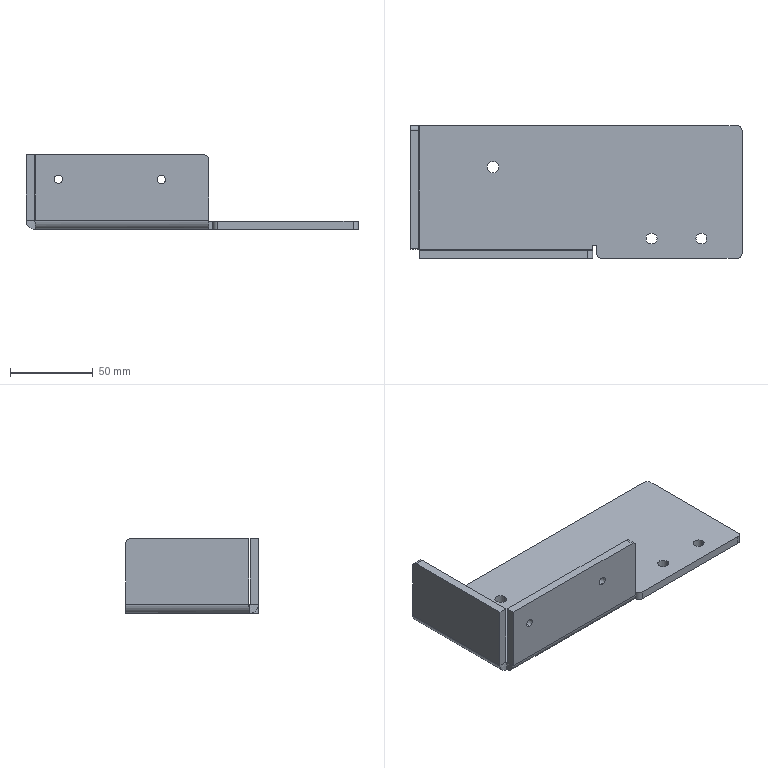Part | SolidWorks | features HoleWzd 3, EdgeFlange 1, Fillet 1, FlatPattern 1, SMBaseFlange 1, SheetMetal 1 | 1 solid | 41 faces | box 200 x 80 x 45 mm | volume 113530 mm3 | plane 20 | cylinder 19 | spline 2 | commonest cylinder face diameters 6 x5 5 x4 6.6 x4 1 x2 7 x2 11 x2
STEP:
#1=CARTESIAN_POINT('',(-18.5,-35.,22.5));
#2=VERTEX_POINT('',#1);
#3=CARTESIAN_POINT('',(-18.5,-35.,27.5));
#4=VERTEX_POINT('',#3);
#5=CARTESIAN_POINT('',(-18.5,-35.,25.));
#6=DIRECTION('',(0.,1.,0.));
#7=DIRECTION('',(0.,0.,1.));
#8=AXIS2_PLACEMENT_3D('',#5,#6,#7);
#9=CIRCLE('',#8,2.5);
#10=EDGE_CURVE('',#2,#4,#9,.T.);
#11=ORIENTED_EDGE('',*,*,#10,.T.);
#12=CARTESIAN_POINT('',(-18.5,-40.,27.5));
#13=VERTEX_POINT('',#12);
#14=CARTESIAN_POINT('',(-18.5,-40.,27.5));
#15=DIRECTION('',(0.,-1.,0.));
#16=VECTOR('',#15,1000.);
#17=LINE('',#14,#16);
#18=EDGE_CURVE('',#4,#13,#17,.T.);
#19=ORIENTED_EDGE('',*,*,#18,.T.);
#20=CARTESIAN_POINT('',(-18.5,-40.,22.5));
#21=VERTEX_POINT('',#20);
#22=CARTESIAN_POINT('',(-18.5,-40.,25.));
#23=DIRECTION('',(0.,-1.,0.));
#24=DIRECTION('',(0.,0.,-1.));
#25=AXIS2_PLACEMENT_3D('',#22,#23,#24);
#26=CIRCLE('',#25,2.5);
#27=EDGE_CURVE('',#13,#21,#26,.T.);
#28=ORIENTED_EDGE('',*,*,#27,.T.);
#29=CARTESIAN_POINT('',(-18.5,-40.,22.5));
#30=DIRECTION('',(0.,-1.,0.));
#31=VECTOR('',#30,1000.);
#32=LINE('',#29,#31);
#33=EDGE_CURVE('',#2,#21,#32,.T.);
#34=ORIENTED_EDGE('',*,*,#33,.F.);
#35=EDGE_LOOP('',(#11,#19,#28,#34));
#36=FACE_OUTER_BOUND('',#35,.T.);
#37=CARTESIAN_POINT('',(-18.5,-40.,25.));
#38=DIRECTION('',(0.,-1.,0.));
#39=DIRECTION('',(0.,0.,-1.));
#40=AXIS2_PLACEMENT_3D('',#37,#38,#39);
#41=CYLINDRICAL_SURFACE('',#40,2.5);
#42=ADVANCED_FACE('',(#36),#41,.F.);
#43=CARTESIAN_POINT('',(-80.5,-35.,22.646));
#44=VERTEX_POINT('',#43);
#45=CARTESIAN_POINT('',(-80.5,-35.,27.646));
#46=VERTEX_POINT('',#45);
#47=CARTESIAN_POINT('',(-80.5,-35.,25.146));
#48=DIRECTION('',(0.,1.,0.));
#49=DIRECTION('',(0.,0.,1.));
#50=AXIS2_PLACEMENT_3D('',#47,#48,#49);
#51=CIRCLE('',#50,2.5);
#52=EDGE_CURVE('',#44,#46,#51,.T.);
#53=ORIENTED_EDGE('',*,*,#52,.T.);
#54=CARTESIAN_POINT('',(-80.5,-40.,27.646));
#55=VERTEX_POINT('',#54);
#56=CARTESIAN_POINT('',(-80.5,-40.,27.646));
#57=DIRECTION('',(0.,-1.,0.));
#58=VECTOR('',#57,1000.);
#59=LINE('',#56,#58);
#60=EDGE_CURVE('',#46,#55,#59,.T.);
#61=ORIENTED_EDGE('',*,*,#60,.T.);
#62=CARTESIAN_POINT('',(-80.5,-40.,22.646));
#63=VERTEX_POINT('',#62);
#64=CARTESIAN_POINT('',(-80.5,-40.,25.146));
#65=DIRECTION('',(0.,-1.,0.));
#66=DIRECTION('',(0.,0.,-1.));
#67=AXIS2_PLACEMENT_3D('',#64,#65,#66);
#68=CIRCLE('',#67,2.5);
#69=EDGE_CURVE('',#55,#63,#68,.T.);
#70=ORIENTED_EDGE('',*,*,#69,.T.);
#71=CARTESIAN_POINT('',(-80.5,-40.,22.646));
#72=DIRECTION('',(0.,-1.,0.));
#73=VECTOR('',#72,1000.);
#74=LINE('',#71,#73);
#75=EDGE_CURVE('',#44,#63,#74,.T.);
#76=ORIENTED_EDGE('',*,*,#75,.F.);
#77=EDGE_LOOP('',(#53,#61,#70,#76));
#78=FACE_OUTER_BOUND('',#77,.T.);
#79=CARTESIAN_POINT('',(-80.5,-40.,25.146));
#80=DIRECTION('',(0.,-1.,0.));
#81=DIRECTION('',(0.,0.,-1.));
#82=AXIS2_PLACEMENT_3D('',#79,#80,#81);
#83=CYLINDRICAL_SURFACE('',#82,2.5);
#84=ADVANCED_FACE('',(#78),#83,.F.);
#85=CARTESIAN_POINT('',(-53.5,15.,-5.));
#86=VERTEX_POINT('',#85);
#87=CARTESIAN_POINT('',(-46.5,15.,-5.));
#88=VERTEX_POINT('',#87);
#89=CARTESIAN_POINT('',(-50.,15.,-5.));
#90=DIRECTION('',(0.,0.,1.));
#91=DIRECTION('',(1.,0.,0.));
#92=AXIS2_PLACEMENT_3D('',#89,#90,#91);
#93=CIRCLE('',#92,3.5);
#94=EDGE_CURVE('',#86,#88,#93,.T.);
#95=ORIENTED_EDGE('',*,*,#94,.F.);
#96=CARTESIAN_POINT('',(-53.5,15.,0.));
#97=VERTEX_POINT('',#96);
#98=CARTESIAN_POINT('',(-53.5,15.,0.));
#99=DIRECTION('',(0.,0.,1.));
#100=VECTOR('',#99,1000.);
#101=LINE('',#98,#100);
#102=EDGE_CURVE('',#86,#97,#101,.T.);
#103=ORIENTED_EDGE('',*,*,#102,.T.);
#104=CARTESIAN_POINT('',(-46.5,15.,0.));
#105=VERTEX_POINT('',#104);
#106=CARTESIAN_POINT('',(-50.,15.,0.));
#107=DIRECTION('',(0.,0.,1.));
#108=DIRECTION('',(1.,0.,0.));
#109=AXIS2_PLACEMENT_3D('',#106,#107,#108);
#110=CIRCLE('',#109,3.5);
#111=EDGE_CURVE('',#97,#105,#110,.T.);
#112=ORIENTED_EDGE('',*,*,#111,.T.);
#113=CARTESIAN_POINT('',(-46.5,15.,0.));
#114=DIRECTION('',(0.,0.,1.));
#115=VECTOR('',#114,1000.);
#116=LINE('',#113,#115);
#117=EDGE_CURVE('',#88,#105,#116,.T.);
#118=ORIENTED_EDGE('',*,*,#117,.F.);
#119=EDGE_LOOP('',(#95,#103,#112,#118));
#120=FACE_OUTER_BOUND('',#119,.T.);
#121=CARTESIAN_POINT('',(-50.,15.,0.));
#122=DIRECTION('',(0.,0.,1.));
#123=DIRECTION('',(1.,0.,0.));
#124=AXIS2_PLACEMENT_3D('',#121,#122,#123);
#125=CYLINDRICAL_SURFACE('',#124,3.5);
#126=ADVANCED_FACE('',(#120),#125,.F.);
#127=CARTESIAN_POINT('',(72.2,-28.,-5.));
#128=VERTEX_POINT('',#127);
#129=CARTESIAN_POINT('',(78.8,-28.,-5.));
#130=VERTEX_POINT('',#129);
#131=CARTESIAN_POINT('',(75.5,-28.,-5.));
#132=DIRECTION('',(0.,0.,1.));
#133=DIRECTION('',(1.,0.,0.));
#134=AXIS2_PLACEMENT_3D('',#131,#132,#133);
#135=CIRCLE('',#134,3.3);
#136=EDGE_CURVE('',#128,#130,#135,.T.);
#137=ORIENTED_EDGE('',*,*,#136,.F.);
#138=CARTESIAN_POINT('',(72.2,-28.,0.));
#139=VERTEX_POINT('',#138);
#140=CARTESIAN_POINT('',(72.2,-28.,0.));
#141=DIRECTION('',(0.,0.,1.));
#142=VECTOR('',#141,1000.);
#143=LINE('',#140,#142);
#144=EDGE_CURVE('',#128,#139,#143,.T.);
#145=ORIENTED_EDGE('',*,*,#144,.T.);
#146=CARTESIAN_POINT('',(78.8,-28.,0.));
#147=VERTEX_POINT('',#146);
#148=CARTESIAN_POINT('',(75.5,-28.,0.));
#149=DIRECTION('',(0.,0.,1.));
#150=DIRECTION('',(1.,0.,0.));
#151=AXIS2_PLACEMENT_3D('',#148,#149,#150);
#152=CIRCLE('',#151,3.3);
#153=EDGE_CURVE('',#139,#147,#152,.T.);
#154=ORIENTED_EDGE('',*,*,#153,.T.);
#155=CARTESIAN_POINT('',(78.8,-28.,0.));
#156=DIRECTION('',(0.,0.,1.));
#157=VECTOR('',#156,1000.);
#158=LINE('',#155,#157);
#159=EDGE_CURVE('',#130,#147,#158,.T.);
#160=ORIENTED_EDGE('',*,*,#159,.F.);
#161=EDGE_LOOP('',(#137,#145,#154,#160));
#162=FACE_OUTER_BOUND('',#161,.T.);
#163=CARTESIAN_POINT('',(75.5,-28.,0.));
#164=DIRECTION('',(0.,0.,1.));
#165=DIRECTION('',(1.,0.,0.));
#166=AXIS2_PLACEMENT_3D('',#163,#164,#165);
#167=CYLINDRICAL_SURFACE('',#166,3.3);
#168=ADVANCED_FACE('',(#162),#167,.F.);
#169=CARTESIAN_POINT('',(42.2,-28.,-5.));
#170=VERTEX_POINT('',#169);
#171=CARTESIAN_POINT('',(48.8,-28.,-5.));
#172=VERTEX_POINT('',#171);
#173=CARTESIAN_POINT('',(45.5,-28.,-5.));
#174=DIRECTION('',(0.,0.,1.));
#175=DIRECTION('',(1.,0.,0.));
#176=AXIS2_PLACEMENT_3D('',#173,#174,#175);
#177=CIRCLE('',#176,3.3);
#178=EDGE_CURVE('',#170,#172,#177,.T.);
#179=ORIENTED_EDGE('',*,*,#178,.F.);
#180=CARTESIAN_POINT('',(42.2,-28.,0.));
#181=VERTEX_POINT('',#180);
#182=CARTESIAN_POINT('',(42.2,-28.,0.));
#183=DIRECTION('',(0.,0.,1.));
#184=VECTOR('',#183,1000.);
#185=LINE('',#182,#184);
#186=EDGE_CURVE('',#170,#181,#185,.T.);
#187=ORIENTED_EDGE('',*,*,#186,.T.);
#188=CARTESIAN_POINT('',(48.8,-28.,0.));
#189=VERTEX_POINT('',#188);
#190=CARTESIAN_POINT('',(45.5,-28.,0.));
#191=DIRECTION('',(0.,0.,1.));
#192=DIRECTION('',(1.,0.,0.));
#193=AXIS2_PLACEMENT_3D('',#190,#191,#192);
#194=CIRCLE('',#193,3.3);
#195=EDGE_CURVE('',#181,#189,#194,.T.);
#196=ORIENTED_EDGE('',*,*,#195,.T.);
#197=CARTESIAN_POINT('',(48.8,-28.,0.));
#198=DIRECTION('',(0.,0.,1.));
#199=VECTOR('',#198,1000.);
#200=LINE('',#197,#199);
#201=EDGE_CURVE('',#172,#189,#200,.T.);
#202=ORIENTED_EDGE('',*,*,#201,.F.);
#203=EDGE_LOOP('',(#179,#187,#196,#202));
#204=FACE_OUTER_BOUND('',#203,.T.);
#205=CARTESIAN_POINT('',(45.5,-28.,0.));
#206=DIRECTION('',(0.,0.,1.));
#207=DIRECTION('',(1.,0.,0.));
#208=AXIS2_PLACEMENT_3D('',#205,#206,#207);
#209=CYLINDRICAL_SURFACE('',#208,3.3);
#210=ADVANCED_FACE('',(#204),#209,.F.);
#211=CARTESIAN_POINT('',(-50.,15.,-5.));
#212=DIRECTION('',(0.,0.,1.));
#213=DIRECTION('',(1.,0.,0.));
#214=AXIS2_PLACEMENT_3D('',#211,#212,#213);
#215=CIRCLE('',#214,3.5);
#216=EDGE_CURVE('',#88,#86,#215,.T.);
#217=ORIENTED_EDGE('',*,*,#216,.T.);
#218=ORIENTED_EDGE('',*,*,#94,.T.);
#219=EDGE_LOOP('',(#217,#218));
#220=FACE_BOUND('',#219,.T.);
#221=CARTESIAN_POINT('',(75.5,-28.,-5.));
#222=DIRECTION('',(0.,0.,1.));
#223=DIRECTION('',(1.,0.,0.));
#224=AXIS2_PLACEMENT_3D('',#221,#222,#223);
#225=CIRCLE('',#224,3.3);
#226=EDGE_CURVE('',#130,#128,#225,.T.);
#227=ORIENTED_EDGE('',*,*,#226,.T.);
#228=ORIENTED_EDGE('',*,*,#136,.T.);
#229=EDGE_LOOP('',(#227,#228));
#230=FACE_BOUND('',#229,.T.);
#231=CARTESIAN_POINT('',(45.5,-28.,-5.));
#232=DIRECTION('',(0.,0.,1.));
#233=DIRECTION('',(1.,0.,0.));
#234=AXIS2_PLACEMENT_3D('',#231,#232,#233);
#235=CIRCLE('',#234,3.3);
#236=EDGE_CURVE('',#172,#170,#235,.T.);
#237=ORIENTED_EDGE('',*,*,#236,.T.);
#238=ORIENTED_EDGE('',*,*,#178,.T.);
#239=EDGE_LOOP('',(#237,#238));
#240=FACE_BOUND('',#239,.T.);
#241=CARTESIAN_POINT('',(15.5,-40.,-5.));
#242=VERTEX_POINT('',#241);
#243=CARTESIAN_POINT('',(97.,-40.,-5.));
#244=VERTEX_POINT('',#243);
#245=CARTESIAN_POINT('',(100.,-40.,-5.));
#246=DIRECTION('',(1.,0.,0.));
#247=VECTOR('',#246,1000.);
#248=LINE('',#245,#247);
#249=EDGE_CURVE('',#242,#244,#248,.T.);
#250=ORIENTED_EDGE('',*,*,#249,.F.);
#251=CARTESIAN_POINT('',(12.5,-37.,-5.));
#252=VERTEX_POINT('',#251);
#253=CARTESIAN_POINT('',(15.5,-37.,-5.));
#254=DIRECTION('',(0.,0.,-1.));
#255=DIRECTION('',(1.,0.,0.));
#256=AXIS2_PLACEMENT_3D('',#253,#254,#255);
#257=CIRCLE('',#256,3.);
#258=EDGE_CURVE('',#242,#252,#257,.T.);
#259=ORIENTED_EDGE('',*,*,#258,.T.);
#260=CARTESIAN_POINT('',(12.5,-32.,-5.));
#261=VERTEX_POINT('',#260);
#262=CARTESIAN_POINT('',(12.5,0.,-5.));
#263=DIRECTION('',(0.,-1.,0.));
#264=VECTOR('',#263,1000.);
#265=LINE('',#262,#264);
#266=EDGE_CURVE('',#261,#252,#265,.T.);
#267=ORIENTED_EDGE('',*,*,#266,.F.);
#268=CARTESIAN_POINT('',(10.,-32.,-5.));
#269=VERTEX_POINT('',#268);
#270=CARTESIAN_POINT('',(0.,-32.,-5.));
#271=DIRECTION('',(1.,0.,0.));
#272=VECTOR('',#271,1000.);
#273=LINE('',#270,#272);
#274=EDGE_CURVE('',#269,#261,#273,.T.);
#275=ORIENTED_EDGE('',*,*,#274,.F.);
#276=CARTESIAN_POINT('',(10.,-34.5,-5.));
#277=VERTEX_POINT('',#276);
#278=CARTESIAN_POINT('',(10.,0.,-5.));
#279=DIRECTION('',(0.,1.,0.));
#280=VECTOR('',#279,1000.);
#281=LINE('',#278,#280);
#282=EDGE_CURVE('',#277,#269,#281,.T.);
#283=ORIENTED_EDGE('',*,*,#282,.F.);
#284=CARTESIAN_POINT('',(-94.5,-34.5,-5.));
#285=VERTEX_POINT('',#284);
#286=CARTESIAN_POINT('',(10.,-34.5,-5.));
#287=DIRECTION('',(-1.,0.,0.));
#288=VECTOR('',#287,1000.);
#289=LINE('',#286,#288);
#290=EDGE_CURVE('',#277,#285,#289,.T.);
#291=ORIENTED_EDGE('',*,*,#290,.T.);
#292=CARTESIAN_POINT('',(-94.5,40.,-5.));
#293=VERTEX_POINT('',#292);
#294=CARTESIAN_POINT('',(-94.5,-34.5,-5.));
#295=DIRECTION('',(0.,1.,0.));
#296=VECTOR('',#295,1000.);
#297=LINE('',#294,#296);
#298=EDGE_CURVE('',#285,#293,#297,.T.);
#299=ORIENTED_EDGE('',*,*,#298,.T.);
#300=CARTESIAN_POINT('',(97.,40.,-5.));
#301=VERTEX_POINT('',#300);
#302=CARTESIAN_POINT('',(100.,40.,-5.));
#303=DIRECTION('',(-1.,0.,0.));
#304=VECTOR('',#303,1000.);
#305=LINE('',#302,#304);
#306=EDGE_CURVE('',#301,#293,#305,.T.);
#307=ORIENTED_EDGE('',*,*,#306,.F.);
#308=CARTESIAN_POINT('',(100.,37.,-5.));
#309=VERTEX_POINT('',#308);
#310=CARTESIAN_POINT('',(97.,37.,-5.));
#311=DIRECTION('',(0.,0.,-1.));
#312=DIRECTION('',(1.,0.,0.));
#313=AXIS2_PLACEMENT_3D('',#310,#311,#312);
#314=CIRCLE('',#313,3.);
#315=EDGE_CURVE('',#301,#309,#314,.T.);
#316=ORIENTED_EDGE('',*,*,#315,.T.);
#317=CARTESIAN_POINT('',(100.,-37.,-5.));
#318=VERTEX_POINT('',#317);
#319=CARTESIAN_POINT('',(100.,-40.,-5.));
#320=DIRECTION('',(0.,1.,0.));
#321=VECTOR('',#320,1000.);
#322=LINE('',#319,#321);
#323=EDGE_CURVE('',#318,#309,#322,.T.);
#324=ORIENTED_EDGE('',*,*,#323,.F.);
#325=CARTESIAN_POINT('',(97.,-37.,-5.));
#326=DIRECTION('',(0.,0.,-1.));
#327=DIRECTION('',(1.,0.,0.));
#328=AXIS2_PLACEMENT_3D('',#325,#326,#327);
#329=CIRCLE('',#328,3.);
#330=EDGE_CURVE('',#318,#244,#329,.T.);
#331=ORIENTED_EDGE('',*,*,#330,.T.);
#332=EDGE_LOOP('',(#250,#259,#267,#275,#283,#291,#299,#307,#316,#324,#331));
#333=FACE_OUTER_BOUND('',#332,.T.);
#334=CARTESIAN_POINT('',(0.,0.,-5.));
#335=DIRECTION('',(0.,0.,1.));
#336=DIRECTION('',(1.,0.,0.));
#337=AXIS2_PLACEMENT_3D('',#334,#335,#336);
#338=PLANE('',#337);
#339=ADVANCED_FACE('',(#220,#230,#240,#333),#338,.F.);
#340=CARTESIAN_POINT('',(-50.,15.,0.));
#341=DIRECTION('',(0.,0.,1.));
#342=DIRECTION('',(1.,0.,0.));
#343=AXIS2_PLACEMENT_3D('',#340,#341,#342);
#344=CIRCLE('',#343,3.5);
#345=EDGE_CURVE('',#105,#97,#344,.T.);
#346=ORIENTED_EDGE('',*,*,#345,.F.);
#347=ORIENTED_EDGE('',*,*,#111,.F.);
#348=EDGE_LOOP('',(#346,#347));
#349=FACE_BOUND('',#348,.T.);
#350=CARTESIAN_POINT('',(75.5,-28.,0.));
#351=DIRECTION('',(0.,0.,1.));
#352=DIRECTION('',(1.,0.,0.));
#353=AXIS2_PLACEMENT_3D('',#350,#351,#352);
#354=CIRCLE('',#353,3.3);
#355=EDGE_CURVE('',#147,#139,#354,.T.);
#356=ORIENTED_EDGE('',*,*,#355,.F.);
#357=ORIENTED_EDGE('',*,*,#153,.F.);
#358=EDGE_LOOP('',(#356,#357));
#359=FACE_BOUND('',#358,.T.);
#360=CARTESIAN_POINT('',(45.5,-28.,0.));
#361=DIRECTION('',(0.,0.,1.));
#362=DIRECTION('',(1.,0.,0.));
#363=AXIS2_PLACEMENT_3D('',#360,#361,#362);
#364=CIRCLE('',#363,3.3);
#365=EDGE_CURVE('',#189,#181,#364,.T.);
#366=ORIENTED_EDGE('',*,*,#365,.F.);
#367=ORIENTED_EDGE('',*,*,#195,.F.);
#368=EDGE_LOOP('',(#366,#367));
#369=FACE_BOUND('',#368,.T.);
#370=CARTESIAN_POINT('',(12.5,-37.,0.));
#371=VERTEX_POINT('',#370);
#372=CARTESIAN_POINT('',(12.5,-32.,0.));
#373=VERTEX_POINT('',#372);
#374=CARTESIAN_POINT('',(12.5,-40.,0.));
#375=DIRECTION('',(0.,1.,0.));
#376=VECTOR('',#375,1000.);
#377=LINE('',#374,#376);
#378=EDGE_CURVE('',#371,#373,#377,.T.);
#379=ORIENTED_EDGE('',*,*,#378,.F.);
#380=CARTESIAN_POINT('',(15.5,-40.,0.));
#381=VERTEX_POINT('',#380);
#382=CARTESIAN_POINT('',(15.5,-37.,0.));
#383=DIRECTION('',(0.,0.,1.));
#384=DIRECTION('',(1.,0.,0.));
#385=AXIS2_PLACEMENT_3D('',#382,#383,#384);
#386=CIRCLE('',#385,3.);
#387=EDGE_CURVE('',#371,#381,#386,.T.);
#388=ORIENTED_EDGE('',*,*,#387,.T.);
#389=CARTESIAN_POINT('',(97.,-40.,0.));
#390=VERTEX_POINT('',#389);
#391=CARTESIAN_POINT('',(100.,-40.,0.));
#392=DIRECTION('',(1.,0.,0.));
#393=VECTOR('',#392,1000.);
#394=LINE('',#391,#393);
#395=EDGE_CURVE('',#381,#390,#394,.T.);
#396=ORIENTED_EDGE('',*,*,#395,.T.);
#397=CARTESIAN_POINT('',(100.,-37.,0.));
#398=VERTEX_POINT('',#397);
#399=CARTESIAN_POINT('',(97.,-37.,0.));
#400=DIRECTION('',(0.,0.,1.));
#401=DIRECTION('',(1.,0.,0.));
#402=AXIS2_PLACEMENT_3D('',#399,#400,#401);
#403=CIRCLE('',#402,3.);
#404=EDGE_CURVE('',#390,#398,#403,.T.);
#405=ORIENTED_EDGE('',*,*,#404,.T.);
#406=CARTESIAN_POINT('',(100.,37.,0.));
#407=VERTEX_POINT('',#406);
#408=CARTESIAN_POINT('',(100.,-40.,0.));
#409=DIRECTION('',(0.,1.,0.));
#410=VECTOR('',#409,1000.);
#411=LINE('',#408,#410);
#412=EDGE_CURVE('',#398,#407,#411,.T.);
#413=ORIENTED_EDGE('',*,*,#412,.T.);
#414=CARTESIAN_POINT('',(97.,40.,0.));
#415=VERTEX_POINT('',#414);
#416=CARTESIAN_POINT('',(97.,37.,0.));
#417=DIRECTION('',(0.,0.,1.));
#418=DIRECTION('',(1.,0.,0.));
#419=AXIS2_PLACEMENT_3D('',#416,#417,#418);
#420=CIRCLE('',#419,3.);
#421=EDGE_CURVE('',#407,#415,#420,.T.);
#422=ORIENTED_EDGE('',*,*,#421,.T.);
#423=CARTESIAN_POINT('',(-94.5,40.,0.));
#424=VERTEX_POINT('',#423);
#425=CARTESIAN_POINT('',(100.,40.,0.));
#426=DIRECTION('',(-1.,0.,0.));
#427=VECTOR('',#426,1000.);
#428=LINE('',#425,#427);
#429=EDGE_CURVE('',#415,#424,#428,.T.);
#430=ORIENTED_EDGE('',*,*,#429,.T.);
#431=CARTESIAN_POINT('',(-94.5,-34.5,0.));
#432=VERTEX_POINT('',#431);
#433=CARTESIAN_POINT('',(-94.5,-34.5,0.));
#434=DIRECTION('',(0.,1.,0.));
#435=VECTOR('',#434,1000.);
#436=LINE('',#433,#435);
#437=EDGE_CURVE('',#432,#424,#436,.T.);
#438=ORIENTED_EDGE('',*,*,#437,.F.);
#439=CARTESIAN_POINT('',(10.,-34.5,0.));
#440=VERTEX_POINT('',#439);
#441=CARTESIAN_POINT('',(10.,-34.5,0.));
#442=DIRECTION('',(-1.,0.,0.));
#443=VECTOR('',#442,1000.);
#444=LINE('',#441,#443);
#445=EDGE_CURVE('',#440,#432,#444,.T.);
#446=ORIENTED_EDGE('',*,*,#445,.F.);
#447=CARTESIAN_POINT('',(10.,-32.,0.));
#448=VERTEX_POINT('',#447);
#449=CARTESIAN_POINT('',(10.,-32.,0.));
#450=DIRECTION('',(0.,-1.,0.));
#451=VECTOR('',#450,1000.);
#452=LINE('',#449,#451);
#453=EDGE_CURVE('',#448,#440,#452,.T.);
#454=ORIENTED_EDGE('',*,*,#453,.F.);
#455=CARTESIAN_POINT('',(12.5,-32.,0.));
#456=DIRECTION('',(-1.,0.,0.));
#457=VECTOR('',#456,1000.);
#458=LINE('',#455,#457);
#459=EDGE_CURVE('',#373,#448,#458,.T.);
#460=ORIENTED_EDGE('',*,*,#459,.F.);
#461=EDGE_LOOP('',(#379,#388,#396,#405,#413,#422,#430,#438,#446,#454,#460));
#462=FACE_OUTER_BOUND('',#461,.T.);
#463=CARTESIAN_POINT('',(0.,0.,0.));
#464=DIRECTION('',(0.,0.,1.));
#465=DIRECTION('',(1.,0.,0.));
#466=AXIS2_PLACEMENT_3D('',#463,#464,#465);
#467=PLANE('',#466);
#468=ADVANCED_FACE('',(#349,#359,#369,#462),#467,.T.);
#469=ORIENTED_EDGE('',*,*,#395,.F.);
#470=CARTESIAN_POINT('',(15.5,-40.,-5.));
#471=DIRECTION('',(0.,0.,-1.));
#472=VECTOR('',#471,1000.);
#473=LINE('',#470,#472);
#474=EDGE_CURVE('',#381,#242,#473,.T.);
#475=ORIENTED_EDGE('',*,*,#474,.T.);
#476=ORIENTED_EDGE('',*,*,#249,.T.);
#477=CARTESIAN_POINT('',(97.,-40.,-5.));
#478=DIRECTION('',(0.,0.,1.));
#479=VECTOR('',#478,1000.);
#480=LINE('',#477,#479);
#481=EDGE_CURVE('',#244,#390,#480,.T.);
#482=ORIENTED_EDGE('',*,*,#481,.T.);
#483=EDGE_LOOP('',(#469,#475,#476,#482));
#484=FACE_OUTER_BOUND('',#483,.T.);
#485=CARTESIAN_POINT('',(100.,-40.,-5.));
#486=DIRECTION('',(0.,-1.,0.));
#487=DIRECTION('',(1.,0.,0.));
#488=AXIS2_PLACEMENT_3D('',#485,#486,#487);
#489=PLANE('',#488);
#490=ADVANCED_FACE('',(#484),#489,.T.);
#491=ORIENTED_EDGE('',*,*,#429,.F.);
#492=CARTESIAN_POINT('',(97.,40.,-5.));
#493=DIRECTION('',(0.,0.,-1.));
#494=VECTOR('',#493,1000.);
#495=LINE('',#492,#494);
#496=EDGE_CURVE('',#415,#301,#495,.T.);
#497=ORIENTED_EDGE('',*,*,#496,.T.);
#498=ORIENTED_EDGE('',*,*,#306,.T.);
#499=CARTESIAN_POINT('',(-94.5,40.,0.));
#500=DIRECTION('',(0.,0.,-1.));
#501=VECTOR('',#500,1000.);
#502=LINE('',#499,#501);
#503=EDGE_CURVE('',#424,#293,#502,.T.);
#504=ORIENTED_EDGE('',*,*,#503,.F.);
#505=EDGE_LOOP('',(#491,#497,#498,#504));
#506=FACE_OUTER_BOUND('',#505,.T.);
#507=CARTESIAN_POINT('',(100.,40.,-5.));
#508=DIRECTION('',(0.,1.,0.));
#509=DIRECTION('',(-1.,0.,0.));
#510=AXIS2_PLACEMENT_3D('',#507,#508,#509);
#511=PLANE('',#510);
#512=ADVANCED_FACE('',(#506),#511,.T.);
#513=ORIENTED_EDGE('',*,*,#323,.T.);
#514=CARTESIAN_POINT('',(100.,37.,-5.));
#515=DIRECTION('',(0.,0.,1.));
#516=VECTOR('',#515,1000.);
#517=LINE('',#514,#516);
#518=EDGE_CURVE('',#309,#407,#517,.T.);
#519=ORIENTED_EDGE('',*,*,#518,.T.);
#520=ORIENTED_EDGE('',*,*,#412,.F.);
#521=CARTESIAN_POINT('',(100.,-37.,-5.));
#522=DIRECTION('',(0.,0.,-1.));
#523=VECTOR('',#522,1000.);
#524=LINE('',#521,#523);
#525=EDGE_CURVE('',#398,#318,#524,.T.);
#526=ORIENTED_EDGE('',*,*,#525,.T.);
#527=EDGE_LOOP('',(#513,#519,#520,#526));
#528=FACE_OUTER_BOUND('',#527,.T.);
#529=CARTESIAN_POINT('',(100.,-40.,-5.));
#530=DIRECTION('',(1.,0.,0.));
#531=DIRECTION('',(0.,0.,-1.));
#532=AXIS2_PLACEMENT_3D('',#529,#530,#531);
#533=PLANE('',#532);
#534=ADVANCED_FACE('',(#528),#533,.T.);
#535=ORIENTED_EDGE('',*,*,#266,.T.);
#536=CARTESIAN_POINT('',(12.5,-37.,0.));
#537=DIRECTION('',(0.,0.,1.));
#538=VECTOR('',#537,1000.);
#539=LINE('',#536,#538);
#540=EDGE_CURVE('',#252,#371,#539,.T.);
#541=ORIENTED_EDGE('',*,*,#540,.T.);
#542=ORIENTED_EDGE('',*,*,#378,.T.);
#543=CARTESIAN_POINT('',(12.5,-32.,0.));
#544=DIRECTION('',(0.,0.,-1.));
#545=VECTOR('',#544,1000.);
#546=LINE('',#543,#545);
#547=EDGE_CURVE('',#373,#261,#546,.T.);
#548=ORIENTED_EDGE('',*,*,#547,.T.);
#549=EDGE_LOOP('',(#535,#541,#542,#548));
#550=FACE_OUTER_BOUND('',#549,.T.);
#551=CARTESIAN_POINT('',(12.5,-40.,0.));
#552=DIRECTION('',(-1.,0.,0.));
#553=DIRECTION('',(0.,-1.,0.));
#554=AXIS2_PLACEMENT_3D('',#551,#552,#553);
#555=PLANE('',#554);
#556=ADVANCED_FACE('',(#550),#555,.T.);
#557=CARTESIAN_POINT('',(10.,-32.,0.));
#558=DIRECTION('',(0.,0.,-1.));
#559=VECTOR('',#558,1000.);
#560=LINE('',#557,#559);
#561=EDGE_CURVE('',#448,#269,#560,.T.);
#562=ORIENTED_EDGE('',*,*,#561,.T.);
#563=ORIENTED_EDGE('',*,*,#274,.T.);
#564=ORIENTED_EDGE('',*,*,#547,.F.);
#565=ORIENTED_EDGE('',*,*,#459,.T.);
#566=EDGE_LOOP('',(#562,#563,#564,#565));
#567=FACE_OUTER_BOUND('',#566,.T.);
#568=CARTESIAN_POINT('',(12.5,-32.,0.));
#569=DIRECTION('',(0.,-1.,0.));
#570=DIRECTION('',(0.,0.,-1.));
#571=AXIS2_PLACEMENT_3D('',#568,#569,#570);
#572=PLANE('',#571);
#573=ADVANCED_FACE('',(#567),#572,.T.);
#574=CARTESIAN_POINT('',(10.,-34.5,0.));
#575=DIRECTION('',(0.,0.,-1.));
#576=VECTOR('',#575,1000.);
#577=LINE('',#574,#576);
#578=EDGE_CURVE('',#440,#277,#577,.T.);
#579=ORIENTED_EDGE('',*,*,#578,.T.);
#580=ORIENTED_EDGE('',*,*,#282,.T.);
#581=ORIENTED_EDGE('',*,*,#561,.F.);
#582=ORIENTED_EDGE('',*,*,#453,.T.);
#583=EDGE_LOOP('',(#579,#580,#581,#582));
#584=FACE_OUTER_BOUND('',#583,.T.);
#585=CARTESIAN_POINT('',(10.,-32.,0.));
#586=DIRECTION('',(1.,0.,0.));
#587=DIRECTION('',(0.,0.,-1.));
#588=AXIS2_PLACEMENT_3D('',#585,#586,#587);
#589=PLANE('',#588);
#590=ADVANCED_FACE('',(#584),#589,.T.);
#591=CARTESIAN_POINT('',(-94.293,-40.,0.5));
#592=VERTEX_POINT('',#591);
#593=CARTESIAN_POINT('',(-94.293,-35.,0.5));
#594=VERTEX_POINT('',#593);
#595=CARTESIAN_POINT('',(-94.293,-35.,0.5));
#596=DIRECTION('',(0.,1.,0.));
#597=VECTOR('',#596,1000.);
#598=LINE('',#595,#597);
#599=EDGE_CURVE('',#592,#594,#598,.T.);
#600=ORIENTED_EDGE('',*,*,#599,.T.);
#601=CARTESIAN_POINT('',(-94.5,-34.5,0.));
#602=CARTESIAN_POINT('',(-94.465,-34.631,0.));
#603=CARTESIAN_POINT('',(-94.431,-34.761,0.05389));
#604=CARTESIAN_POINT('',(-94.362,-34.946,0.239));
#605=CARTESIAN_POINT('',(-94.327,-35.,0.3691));
#606=CARTESIAN_POINT('',(-94.293,-35.,0.5));
#607=B_SPLINE_CURVE_WITH_KNOTS('',3,(#601,#602,#603,#604,#605,#606),.UNSPECIFIED.,.F.,.F.,(4,2,4),(0.,0.5,1.),.UNSPECIFIED.);
#608=EDGE_CURVE('',#432,#594,#607,.T.);
#609=ORIENTED_EDGE('',*,*,#608,.F.);
#610=CARTESIAN_POINT('',(-94.5,-34.5,0.));
#611=DIRECTION('',(0.,0.,-1.));
#612=VECTOR('',#611,1000.);
#613=LINE('',#610,#612);
#614=EDGE_CURVE('',#432,#285,#613,.T.);
#615=ORIENTED_EDGE('',*,*,#614,.T.);
#616=CARTESIAN_POINT('',(-94.5,-34.5,-5.));
#617=CARTESIAN_POINT('',(-94.483,-35.22,-5.));
#618=CARTESIAN_POINT('',(-94.465,-35.94,-4.857));
#619=CARTESIAN_POINT('',(-94.431,-37.27,-4.306));
#620=CARTESIAN_POINT('',(-94.414,-37.88,-3.898));
#621=CARTESIAN_POINT('',(-94.379,-38.898,-2.88));
#622=CARTESIAN_POINT('',(-94.362,-39.306,-2.27));
#623=CARTESIAN_POINT('',(-94.327,-39.857,-0.9396));
#624=CARTESIAN_POINT('',(-94.31,-40.,-0.2199));
#625=CARTESIAN_POINT('',(-94.293,-40.,0.5));
#626=B_SPLINE_CURVE_WITH_KNOTS('',3,(#616,#617,#618,#619,#620,#621,#622,#623,#624,#625),.UNSPECIFIED.,.F.,.F.,(4,2,2,2,4),(0.,0.25,0.5,0.75,1.),.UNSPECIFIED.);
#627=EDGE_CURVE('',#285,#592,#626,.T.);
#628=ORIENTED_EDGE('',*,*,#627,.T.);
#629=EDGE_LOOP('',(#600,#609,#615,#628));
#630=FACE_OUTER_BOUND('',#629,.T.);
#631=CARTESIAN_POINT('',(-94.5,-34.5,-5.05));
#632=CARTESIAN_POINT('',(-94.483,-35.227,-5.05));
#633=CARTESIAN_POINT('',(-94.465,-35.953,-4.906));
#634=CARTESIAN_POINT('',(-94.431,-37.295,-4.35));
#635=CARTESIAN_POINT('',(-94.414,-37.911,-3.938));
#636=CARTESIAN_POINT('',(-94.379,-38.938,-2.911));
#637=CARTESIAN_POINT('',(-94.362,-39.35,-2.295));
#638=CARTESIAN_POINT('',(-94.327,-39.906,-0.9527));
#639=CARTESIAN_POINT('',(-94.31,-40.05,-0.2266));
#640=CARTESIAN_POINT('',(-94.293,-40.05,0.5));
#641=CARTESIAN_POINT('',(-94.5,-34.5,-5.));
#642=CARTESIAN_POINT('',(-94.483,-35.22,-5.));
#643=CARTESIAN_POINT('',(-94.465,-35.94,-4.857));
#644=CARTESIAN_POINT('',(-94.431,-37.27,-4.306));
#645=CARTESIAN_POINT('',(-94.414,-37.88,-3.898));
#646=CARTESIAN_POINT('',(-94.379,-38.898,-2.88));
#647=CARTESIAN_POINT('',(-94.362,-39.306,-2.27));
#648=CARTESIAN_POINT('',(-94.327,-39.857,-0.9396));
#649=CARTESIAN_POINT('',(-94.31,-40.,-0.2201));
#650=CARTESIAN_POINT('',(-94.293,-40.,0.5));
#651=CARTESIAN_POINT('',(-94.5,-34.5,0.));
#652=CARTESIAN_POINT('',(-94.483,-34.565,0.));
#653=CARTESIAN_POINT('',(-94.465,-34.631,0.01301));
#654=CARTESIAN_POINT('',(-94.431,-34.752,0.06311));
#655=CARTESIAN_POINT('',(-94.414,-34.807,0.1002));
#656=CARTESIAN_POINT('',(-94.379,-34.9,0.1927));
#657=CARTESIAN_POINT('',(-94.362,-34.937,0.2482));
#658=CARTESIAN_POINT('',(-94.327,-34.987,0.3691));
#659=CARTESIAN_POINT('',(-94.31,-35.,0.4345));
#660=CARTESIAN_POINT('',(-94.293,-35.,0.5));
#661=CARTESIAN_POINT('',(-94.5,-34.5,0.0505));
#662=CARTESIAN_POINT('',(-94.483,-34.559,0.0505));
#663=CARTESIAN_POINT('',(-94.465,-34.618,0.0622));
#664=CARTESIAN_POINT('',(-94.431,-34.726,0.1072));
#665=CARTESIAN_POINT('',(-94.414,-34.776,0.1405));
#666=CARTESIAN_POINT('',(-94.379,-34.859,0.2238));
#667=CARTESIAN_POINT('',(-94.362,-34.893,0.2736));
#668=CARTESIAN_POINT('',(-94.327,-34.938,0.3823));
#669=CARTESIAN_POINT('',(-94.31,-34.95,0.4412));
#670=CARTESIAN_POINT('',(-94.293,-34.95,0.5));
#671=B_SPLINE_SURFACE_WITH_KNOTS('',1,3,((#631,#632,#633,#634,#635,#636,#637,#638,#639,#640),(#641,#642,#643,#644,#645,#646,#647,#648,#649,#650),(#651,#652,#653,#654,#655,#656,#657,#658,#659,#660),(#661,#662,#663,#664,#665,#666,#667,#668,#669,#670)),.UNSPECIFIED.,.F.,.F.,.F.,(2,1,1,2),(4,2,2,2,4),(-0.01,0.,1.,1.01),(0.,0.25,0.5,0.75,1.),.UNSPECIFIED.);
#672=ADVANCED_FACE('',(#630),#671,.F.);
#673=CARTESIAN_POINT('',(10.,-35.,0.5));
#674=VERTEX_POINT('',#673);
#675=CARTESIAN_POINT('',(10.,-34.5,0.5));
#676=DIRECTION('',(1.,0.,0.));
#677=DIRECTION('',(0.,0.,-1.));
#678=AXIS2_PLACEMENT_3D('',#675,#676,#677);
#679=CIRCLE('',#678,0.5);
#680=EDGE_CURVE('',#674,#440,#679,.T.);
#681=ORIENTED_EDGE('',*,*,#680,.F.);
#682=CARTESIAN_POINT('',(10.,-40.,0.5));
#683=VERTEX_POINT('',#682);
#684=CARTESIAN_POINT('',(10.,-35.,0.5));
#685=DIRECTION('',(0.,-1.,0.));
#686=VECTOR('',#685,1000.);
#687=LINE('',#684,#686);
#688=EDGE_CURVE('',#674,#683,#687,.T.);
#689=ORIENTED_EDGE('',*,*,#688,.T.);
#690=CARTESIAN_POINT('',(10.,-34.5,0.5));
#691=DIRECTION('',(1.,0.,0.));
#692=DIRECTION('',(0.,0.,-1.));
#693=AXIS2_PLACEMENT_3D('',#690,#691,#692);
#694=CIRCLE('',#693,5.5);
#695=EDGE_CURVE('',#683,#277,#694,.T.);
#696=ORIENTED_EDGE('',*,*,#695,.T.);
#697=ORIENTED_EDGE('',*,*,#578,.F.);
#698=EDGE_LOOP('',(#681,#689,#696,#697));
#699=FACE_OUTER_BOUND('',#698,.T.);
#700=CARTESIAN_POINT('',(10.,-34.5,0.5));
#701=DIRECTION('',(-1.,0.,0.));
#702=DIRECTION('',(0.,0.,1.));
#703=AXIS2_PLACEMENT_3D('',#700,#701,#702);
#704=PLANE('',#703);
#705=ADVANCED_FACE('',(#699),#704,.F.);
#706=ORIENTED_EDGE('',*,*,#290,.F.);
#707=ORIENTED_EDGE('',*,*,#695,.F.);
#708=CARTESIAN_POINT('',(-100.,-40.,0.5));
#709=DIRECTION('',(-1.,0.,0.));
#710=VECTOR('',#709,1000.);
#711=LINE('',#708,#710);
#712=EDGE_CURVE('',#683,#592,#711,.T.);
#713=ORIENTED_EDGE('',*,*,#712,.T.);
#714=ORIENTED_EDGE('',*,*,#627,.F.);
#715=EDGE_LOOP('',(#706,#707,#713,#714));
#716=FACE_OUTER_BOUND('',#715,.T.);
#717=CARTESIAN_POINT('',(10.,-34.5,0.5));
#718=DIRECTION('',(1.,0.,0.));
#719=DIRECTION('',(0.,-1.,0.));
#720=AXIS2_PLACEMENT_3D('',#717,#718,#719);
#721=CYLINDRICAL_SURFACE('',#720,5.5);
#722=ADVANCED_FACE('',(#716),#721,.T.);
#723=ORIENTED_EDGE('',*,*,#445,.T.);
#724=ORIENTED_EDGE('',*,*,#608,.T.);
#725=CARTESIAN_POINT('',(-100.,-35.,0.5));
#726=DIRECTION('',(1.,0.,0.));
#727=VECTOR('',#726,1000.);
#728=LINE('',#725,#727);
#729=EDGE_CURVE('',#594,#674,#728,.T.);
#730=ORIENTED_EDGE('',*,*,#729,.T.);
#731=ORIENTED_EDGE('',*,*,#680,.T.);
#732=EDGE_LOOP('',(#723,#724,#730,#731));
#733=FACE_OUTER_BOUND('',#732,.T.);
#734=CARTESIAN_POINT('',(10.,-34.5,0.5));
#735=DIRECTION('',(1.,0.,0.));
#736=DIRECTION('',(0.,-1.,0.));
#737=AXIS2_PLACEMENT_3D('',#734,#735,#736);
#738=CYLINDRICAL_SURFACE('',#737,0.5);
#739=ADVANCED_FACE('',(#733),#738,.F.);
#740=CARTESIAN_POINT('',(-94.293,-40.,40.));
#741=VERTEX_POINT('',#740);
#742=CARTESIAN_POINT('',(-94.293,-40.,0.));
#743=DIRECTION('',(0.,0.,1.));
#744=VECTOR('',#743,1000.);
#745=LINE('',#742,#744);
#746=EDGE_CURVE('',#592,#741,#745,.T.);
#747=ORIENTED_EDGE('',*,*,#746,.T.);
#748=CARTESIAN_POINT('',(-94.293,-35.,40.));
#749=VERTEX_POINT('',#748);
#750=CARTESIAN_POINT('',(-94.293,-35.,40.));
#751=DIRECTION('',(0.,1.,0.));
#752=VECTOR('',#751,1000.);
#753=LINE('',#750,#752);
#754=EDGE_CURVE('',#741,#749,#753,.T.);
#755=ORIENTED_EDGE('',*,*,#754,.T.);
#756=CARTESIAN_POINT('',(-94.293,-35.,0.));
#757=DIRECTION('',(0.,0.,1.));
#758=VECTOR('',#757,1000.);
#759=LINE('',#756,#758);
#760=EDGE_CURVE('',#594,#749,#759,.T.);
#761=ORIENTED_EDGE('',*,*,#760,.F.);
#762=ORIENTED_EDGE('',*,*,#599,.F.);
#763=EDGE_LOOP('',(#747,#755,#761,#762));
#764=FACE_OUTER_BOUND('',#763,.T.);
#765=CARTESIAN_POINT('',(-94.293,-35.,0.));
#766=DIRECTION('',(-1.,0.,0.));
#767=DIRECTION('',(0.,0.,1.));
#768=AXIS2_PLACEMENT_3D('',#765,#766,#767);
#769=PLANE('',#768);
#770=ADVANCED_FACE('',(#764),#769,.T.);
#771=CARTESIAN_POINT('',(-18.5,-40.,25.));
#772=DIRECTION('',(0.,-1.,0.));
#773=DIRECTION('',(0.,0.,-1.));
#774=AXIS2_PLACEMENT_3D('',#771,#772,#773);
#775=CIRCLE('',#774,2.5);
#776=EDGE_CURVE('',#21,#13,#775,.T.);
#777=ORIENTED_EDGE('',*,*,#776,.F.);
#778=ORIENTED_EDGE('',*,*,#27,.F.);
#779=EDGE_LOOP('',(#777,#778));
#780=FACE_BOUND('',#779,.T.);
#781=CARTESIAN_POINT('',(-80.5,-40.,25.146));
#782=DIRECTION('',(0.,-1.,0.));
#783=DIRECTION('',(0.,0.,-1.));
#784=AXIS2_PLACEMENT_3D('',#781,#782,#783);
#785=CIRCLE('',#784,2.5);
#786=EDGE_CURVE('',#63,#55,#785,.T.);
#787=ORIENTED_EDGE('',*,*,#786,.F.);
#788=ORIENTED_EDGE('',*,*,#69,.F.);
#789=EDGE_LOOP('',(#787,#788));
#790=FACE_BOUND('',#789,.T.);
#791=CARTESIAN_POINT('',(10.,-40.,37.));
#792=VERTEX_POINT('',#791);
#793=CARTESIAN_POINT('',(10.,-40.,0.));
#794=DIRECTION('',(0.,0.,1.));
#795=VECTOR('',#794,1000.);
#796=LINE('',#793,#795);
#797=EDGE_CURVE('',#683,#792,#796,.T.);
#798=ORIENTED_EDGE('',*,*,#797,.T.);
#799=CARTESIAN_POINT('',(7.,-40.,40.));
#800=VERTEX_POINT('',#799);
#801=CARTESIAN_POINT('',(7.,-40.,37.));
#802=DIRECTION('',(0.,-1.,0.));
#803=DIRECTION('',(0.,0.,1.));
#804=AXIS2_PLACEMENT_3D('',#801,#802,#803);
#805=CIRCLE('',#804,3.);
#806=EDGE_CURVE('',#792,#800,#805,.T.);
#807=ORIENTED_EDGE('',*,*,#806,.T.);
#808=CARTESIAN_POINT('',(0.,-40.,40.));
#809=DIRECTION('',(-1.,0.,0.));
#810=VECTOR('',#809,1000.);
#811=LINE('',#808,#810);
#812=EDGE_CURVE('',#800,#741,#811,.T.);
#813=ORIENTED_EDGE('',*,*,#812,.T.);
#814=ORIENTED_EDGE('',*,*,#746,.F.);
#815=ORIENTED_EDGE('',*,*,#712,.F.);
#816=EDGE_LOOP('',(#798,#807,#813,#814,#815));
#817=FACE_OUTER_BOUND('',#816,.T.);
#818=CARTESIAN_POINT('',(0.,-40.,0.));
#819=DIRECTION('',(0.,1.,0.));
#820=DIRECTION('',(0.,0.,1.));
#821=AXIS2_PLACEMENT_3D('',#818,#819,#820);
#822=PLANE('',#821);
#823=ADVANCED_FACE('',(#780,#790,#817),#822,.F.);
#824=ORIENTED_EDGE('',*,*,#10,.F.);
#825=CARTESIAN_POINT('',(-18.5,-35.,25.));
#826=DIRECTION('',(0.,1.,0.));
#827=DIRECTION('',(0.,0.,1.));
#828=AXIS2_PLACEMENT_3D('',#825,#826,#827);
#829=CIRCLE('',#828,2.5);
#830=EDGE_CURVE('',#4,#2,#829,.T.);
#831=ORIENTED_EDGE('',*,*,#830,.F.);
#832=EDGE_LOOP('',(#824,#831));
#833=FACE_BOUND('',#832,.T.);
#834=ORIENTED_EDGE('',*,*,#52,.F.);
#835=CARTESIAN_POINT('',(-80.5,-35.,25.146));
#836=DIRECTION('',(0.,1.,0.));
#837=DIRECTION('',(0.,0.,1.));
#838=AXIS2_PLACEMENT_3D('',#835,#836,#837);
#839=CIRCLE('',#838,2.5);
#840=EDGE_CURVE('',#46,#44,#839,.T.);
#841=ORIENTED_EDGE('',*,*,#840,.F.);
#842=EDGE_LOOP('',(#834,#841));
#843=FACE_BOUND('',#842,.T.);
#844=CARTESIAN_POINT('',(7.,-35.,40.));
#845=VERTEX_POINT('',#844);
#846=CARTESIAN_POINT('',(-100.,-35.,40.));
#847=DIRECTION('',(-1.,0.,0.));
#848=VECTOR('',#847,1000.);
#849=LINE('',#846,#848);
#850=EDGE_CURVE('',#845,#749,#849,.T.);
#851=ORIENTED_EDGE('',*,*,#850,.F.);
#852=CARTESIAN_POINT('',(10.,-35.,37.));
#853=VERTEX_POINT('',#852);
#854=CARTESIAN_POINT('',(7.,-35.,37.));
#855=DIRECTION('',(0.,1.,0.));
#856=DIRECTION('',(0.,0.,1.));
#857=AXIS2_PLACEMENT_3D('',#854,#855,#856);
#858=CIRCLE('',#857,3.);
#859=EDGE_CURVE('',#845,#853,#858,.T.);
#860=ORIENTED_EDGE('',*,*,#859,.T.);
#861=CARTESIAN_POINT('',(10.,-35.,40.));
#862=DIRECTION('',(0.,0.,1.));
#863=VECTOR('',#862,1000.);
#864=LINE('',#861,#863);
#865=EDGE_CURVE('',#674,#853,#864,.T.);
#866=ORIENTED_EDGE('',*,*,#865,.F.);
#867=ORIENTED_EDGE('',*,*,#729,.F.);
#868=ORIENTED_EDGE('',*,*,#760,.T.);
#869=EDGE_LOOP('',(#851,#860,#866,#867,#868));
#870=FACE_OUTER_BOUND('',#869,.T.);
#871=CARTESIAN_POINT('',(0.,-35.,0.));
#872=DIRECTION('',(0.,1.,0.));
#873=DIRECTION('',(0.,0.,1.));
#874=AXIS2_PLACEMENT_3D('',#871,#872,#873);
#875=PLANE('',#874);
#876=ADVANCED_FACE('',(#833,#843,#870),#875,.T.);
#877=ORIENTED_EDGE('',*,*,#812,.F.);
#878=CARTESIAN_POINT('',(7.,-40.,40.));
#879=DIRECTION('',(0.,1.,0.));
#880=VECTOR('',#879,1000.);
#881=LINE('',#878,#880);
#882=EDGE_CURVE('',#800,#845,#881,.T.);
#883=ORIENTED_EDGE('',*,*,#882,.T.);
#884=ORIENTED_EDGE('',*,*,#850,.T.);
#885=ORIENTED_EDGE('',*,*,#754,.F.);
#886=EDGE_LOOP('',(#877,#883,#884,#885));
#887=FACE_OUTER_BOUND('',#886,.T.);
#888=CARTESIAN_POINT('',(-100.,-40.,40.));
#889=DIRECTION('',(0.,0.,-1.));
#890=DIRECTION('',(0.,1.,0.));
#891=AXIS2_PLACEMENT_3D('',#888,#889,#890);
#892=PLANE('',#891);
#893=ADVANCED_FACE('',(#887),#892,.F.);
#894=ORIENTED_EDGE('',*,*,#865,.T.);
#895=CARTESIAN_POINT('',(10.,-40.,37.));
#896=DIRECTION('',(0.,-1.,0.));
#897=VECTOR('',#896,1000.);
#898=LINE('',#895,#897);
#899=EDGE_CURVE('',#853,#792,#898,.T.);
#900=ORIENTED_EDGE('',*,*,#899,.T.);
#901=ORIENTED_EDGE('',*,*,#797,.F.);
#902=ORIENTED_EDGE('',*,*,#688,.F.);
#903=EDGE_LOOP('',(#894,#900,#901,#902));
#904=FACE_OUTER_BOUND('',#903,.T.);
#905=CARTESIAN_POINT('',(10.,-40.,40.));
#906=DIRECTION('',(-1.,0.,0.));
#907=DIRECTION('',(0.,-1.,0.));
#908=AXIS2_PLACEMENT_3D('',#905,#906,#907);
#909=PLANE('',#908);
#910=ADVANCED_FACE('',(#904),#909,.F.);
#911=CARTESIAN_POINT('',(-95.,40.,0.5));
#912=VERTEX_POINT('',#911);
#913=CARTESIAN_POINT('',(-100.,40.,0.5));
#914=VERTEX_POINT('',#913);
#915=CARTESIAN_POINT('',(-100.,40.,0.5));
#916=DIRECTION('',(-1.,0.,0.));
#917=VECTOR('',#916,1000.);
#918=LINE('',#915,#917);
#919=EDGE_CURVE('',#912,#914,#918,.T.);
#920=ORIENTED_EDGE('',*,*,#919,.F.);
#921=CARTESIAN_POINT('',(-94.5,40.,0.5));
#922=DIRECTION('',(0.,1.,0.));
#923=DIRECTION('',(0.,0.,-1.));
#924=AXIS2_PLACEMENT_3D('',#921,#922,#923);
#925=CIRCLE('',#924,0.5);
#926=EDGE_CURVE('',#424,#912,#925,.T.);
#927=ORIENTED_EDGE('',*,*,#926,.F.);
#928=ORIENTED_EDGE('',*,*,#503,.T.);
#929=CARTESIAN_POINT('',(-94.5,40.,0.5));
#930=DIRECTION('',(0.,1.,0.));
#931=DIRECTION('',(0.,0.,-1.));
#932=AXIS2_PLACEMENT_3D('',#929,#930,#931);
#933=CIRCLE('',#932,5.5);
#934=EDGE_CURVE('',#293,#914,#933,.T.);
#935=ORIENTED_EDGE('',*,*,#934,.T.);
#936=EDGE_LOOP('',(#920,#927,#928,#935));
#937=FACE_OUTER_BOUND('',#936,.T.);
#938=CARTESIAN_POINT('',(-94.5,40.,0.5));
#939=DIRECTION('',(0.,1.,0.));
#940=DIRECTION('',(0.,0.,1.));
#941=AXIS2_PLACEMENT_3D('',#938,#939,#940);
#942=PLANE('',#941);
#943=ADVANCED_FACE('',(#937),#942,.T.);
#944=CARTESIAN_POINT('',(-95.,-34.293,0.5));
#945=VERTEX_POINT('',#944);
#946=CARTESIAN_POINT('',(-95.,-34.293,0.5));
#947=CARTESIAN_POINT('',(-95.,-34.327,0.3691));
#948=CARTESIAN_POINT('',(-94.946,-34.362,0.239));
#949=CARTESIAN_POINT('',(-94.761,-34.431,0.05389));
#950=CARTESIAN_POINT('',(-94.631,-34.465,0.));
#951=CARTESIAN_POINT('',(-94.5,-34.5,0.));
#952=B_SPLINE_CURVE_WITH_KNOTS('',3,(#946,#947,#948,#949,#950,#951),.UNSPECIFIED.,.F.,.F.,(4,2,4),(0.,0.5,1.),.UNSPECIFIED.);
#953=EDGE_CURVE('',#945,#432,#952,.T.);
#954=ORIENTED_EDGE('',*,*,#953,.F.);
#955=CARTESIAN_POINT('',(-100.,-34.293,0.5));
#956=VERTEX_POINT('',#955);
#957=CARTESIAN_POINT('',(-95.,-34.293,0.5));
#958=DIRECTION('',(1.,0.,0.));
#959=VECTOR('',#958,1000.);
#960=LINE('',#957,#959);
#961=EDGE_CURVE('',#956,#945,#960,.T.);
#962=ORIENTED_EDGE('',*,*,#961,.F.);
#963=CARTESIAN_POINT('',(-100.,-34.293,0.5));
#964=CARTESIAN_POINT('',(-100.,-34.31,-0.2199));
#965=CARTESIAN_POINT('',(-99.857,-34.327,-0.9396));
#966=CARTESIAN_POINT('',(-99.306,-34.362,-2.27));
#967=CARTESIAN_POINT('',(-98.898,-34.379,-2.88));
#968=CARTESIAN_POINT('',(-97.88,-34.414,-3.898));
#969=CARTESIAN_POINT('',(-97.27,-34.431,-4.306));
#970=CARTESIAN_POINT('',(-95.94,-34.465,-4.857));
#971=CARTESIAN_POINT('',(-95.22,-34.483,-5.));
#972=CARTESIAN_POINT('',(-94.5,-34.5,-5.));
#973=B_SPLINE_CURVE_WITH_KNOTS('',3,(#963,#964,#965,#966,#967,#968,#969,#970,#971,#972),.UNSPECIFIED.,.F.,.F.,(4,2,2,2,4),(0.,0.25,0.5,0.75,1.),.UNSPECIFIED.);
#974=EDGE_CURVE('',#956,#285,#973,.T.);
#975=ORIENTED_EDGE('',*,*,#974,.T.);
#976=ORIENTED_EDGE('',*,*,#614,.F.);
#977=EDGE_LOOP('',(#954,#962,#975,#976));
#978=FACE_OUTER_BOUND('',#977,.T.);
#979=CARTESIAN_POINT('',(-100.05,-34.293,0.5));
#980=CARTESIAN_POINT('',(-100.05,-34.31,-0.2266));
#981=CARTESIAN_POINT('',(-99.906,-34.327,-0.9527));
#982=CARTESIAN_POINT('',(-99.35,-34.362,-2.295));
#983=CARTESIAN_POINT('',(-98.938,-34.379,-2.911));
#984=CARTESIAN_POINT('',(-97.911,-34.414,-3.938));
#985=CARTESIAN_POINT('',(-97.295,-34.431,-4.35));
#986=CARTESIAN_POINT('',(-95.953,-34.465,-4.906));
#987=CARTESIAN_POINT('',(-95.227,-34.483,-5.05));
#988=CARTESIAN_POINT('',(-94.5,-34.5,-5.05));
#989=CARTESIAN_POINT('',(-100.,-34.293,0.5));
#990=CARTESIAN_POINT('',(-100.,-34.31,-0.2201));
#991=CARTESIAN_POINT('',(-99.857,-34.327,-0.9396));
#992=CARTESIAN_POINT('',(-99.306,-34.362,-2.27));
#993=CARTESIAN_POINT('',(-98.898,-34.379,-2.88));
#994=CARTESIAN_POINT('',(-97.88,-34.414,-3.898));
#995=CARTESIAN_POINT('',(-97.27,-34.431,-4.306));
#996=CARTESIAN_POINT('',(-95.94,-34.465,-4.857));
#997=CARTESIAN_POINT('',(-95.22,-34.483,-5.));
#998=CARTESIAN_POINT('',(-94.5,-34.5,-5.));
#999=CARTESIAN_POINT('',(-95.,-34.293,0.5));
#1000=CARTESIAN_POINT('',(-95.,-34.31,0.4345));
#1001=CARTESIAN_POINT('',(-94.987,-34.327,0.3691));
#1002=CARTESIAN_POINT('',(-94.937,-34.362,0.2482));
#1003=CARTESIAN_POINT('',(-94.9,-34.379,0.1927));
#1004=CARTESIAN_POINT('',(-94.807,-34.414,0.1002));
#1005=CARTESIAN_POINT('',(-94.752,-34.431,0.06311));
#1006=CARTESIAN_POINT('',(-94.631,-34.465,0.01301));
#1007=CARTESIAN_POINT('',(-94.565,-34.483,0.));
#1008=CARTESIAN_POINT('',(-94.5,-34.5,0.));
#1009=CARTESIAN_POINT('',(-94.95,-34.293,0.5));
#1010=CARTESIAN_POINT('',(-94.95,-34.31,0.4412));
#1011=CARTESIAN_POINT('',(-94.938,-34.327,0.3823));
#1012=CARTESIAN_POINT('',(-94.893,-34.362,0.2736));
#1013=CARTESIAN_POINT('',(-94.859,-34.379,0.2238));
#1014=CARTESIAN_POINT('',(-94.776,-34.414,0.1405));
#1015=CARTESIAN_POINT('',(-94.726,-34.431,0.1072));
#1016=CARTESIAN_POINT('',(-94.618,-34.465,0.0622));
#1017=CARTESIAN_POINT('',(-94.559,-34.483,0.0505));
#1018=CARTESIAN_POINT('',(-94.5,-34.5,0.0505));
#1019=B_SPLINE_SURFACE_WITH_KNOTS('',1,3,((#979,#980,#981,#982,#983,#984,#985,#986,#987,#988),(#989,#990,#991,#992,#993,#994,#995,#996,#997,#998),(#999,#1000,#1001,#1002,#1003,#1004,#1005,#1006,#1007,#1008),(#1009,#1010,#1011,#1012,#1013,#1014,#1015,#1016,#1017,#1018)),.UNSPECIFIED.,.F.,.F.,.F.,(2,1,1,2),(4,2,2,2,4),(-0.01,0.,1.,1.01),(0.,0.25,0.5,0.75,1.),.UNSPECIFIED.);
#1020=ADVANCED_FACE('',(#978),#1019,.F.);
#1021=ORIENTED_EDGE('',*,*,#298,.F.);
#1022=ORIENTED_EDGE('',*,*,#974,.F.);
#1023=CARTESIAN_POINT('',(-100.,40.,0.5));
#1024=DIRECTION('',(0.,1.,0.));
#1025=VECTOR('',#1024,1000.);
#1026=LINE('',#1023,#1025);
#1027=EDGE_CURVE('',#956,#914,#1026,.T.);
#1028=ORIENTED_EDGE('',*,*,#1027,.T.);
#1029=ORIENTED_EDGE('',*,*,#934,.F.);
#1030=EDGE_LOOP('',(#1021,#1022,#1028,#1029));
#1031=FACE_OUTER_BOUND('',#1030,.T.);
#1032=CARTESIAN_POINT('',(-94.5,-34.5,0.5));
#1033=DIRECTION('',(0.,-1.,0.));
#1034=DIRECTION('',(-1.,0.,0.));
#1035=AXIS2_PLACEMENT_3D('',#1032,#1033,#1034);
#1036=CYLINDRICAL_SURFACE('',#1035,5.5);
#1037=ADVANCED_FACE('',(#1031),#1036,.T.);
#1038=ORIENTED_EDGE('',*,*,#437,.T.);
#1039=ORIENTED_EDGE('',*,*,#926,.T.);
#1040=CARTESIAN_POINT('',(-95.,40.,0.5));
#1041=DIRECTION('',(0.,-1.,0.));
#1042=VECTOR('',#1041,1000.);
#1043=LINE('',#1040,#1042);
#1044=EDGE_CURVE('',#912,#945,#1043,.T.);
#1045=ORIENTED_EDGE('',*,*,#1044,.T.);
#1046=ORIENTED_EDGE('',*,*,#953,.T.);
#1047=EDGE_LOOP('',(#1038,#1039,#1045,#1046));
#1048=FACE_OUTER_BOUND('',#1047,.T.);
#1049=CARTESIAN_POINT('',(-94.5,-34.5,0.5));
#1050=DIRECTION('',(0.,-1.,0.));
#1051=DIRECTION('',(-1.,0.,0.));
#1052=AXIS2_PLACEMENT_3D('',#1049,#1050,#1051);
#1053=CYLINDRICAL_SURFACE('',#1052,0.5);
#1054=ADVANCED_FACE('',(#1048),#1053,.F.);
#1055=CARTESIAN_POINT('',(-100.,40.,37.));
#1056=VERTEX_POINT('',#1055);
#1057=CARTESIAN_POINT('',(-100.,40.,0.));
#1058=DIRECTION('',(0.,0.,-1.));
#1059=VECTOR('',#1058,1000.);
#1060=LINE('',#1057,#1059);
#1061=EDGE_CURVE('',#1056,#914,#1060,.T.);
#1062=ORIENTED_EDGE('',*,*,#1061,.F.);
#1063=CARTESIAN_POINT('',(-95.,40.,37.));
#1064=VERTEX_POINT('',#1063);
#1065=CARTESIAN_POINT('',(-100.,40.,37.));
#1066=DIRECTION('',(1.,0.,0.));
#1067=VECTOR('',#1066,1000.);
#1068=LINE('',#1065,#1067);
#1069=EDGE_CURVE('',#1056,#1064,#1068,.T.);
#1070=ORIENTED_EDGE('',*,*,#1069,.T.);
#1071=CARTESIAN_POINT('',(-95.,40.,0.));
#1072=DIRECTION('',(0.,0.,-1.));
#1073=VECTOR('',#1072,1000.);
#1074=LINE('',#1071,#1073);
#1075=EDGE_CURVE('',#1064,#912,#1074,.T.);
#1076=ORIENTED_EDGE('',*,*,#1075,.T.);
#1077=ORIENTED_EDGE('',*,*,#919,.T.);
#1078=EDGE_LOOP('',(#1062,#1070,#1076,#1077));
#1079=FACE_OUTER_BOUND('',#1078,.T.);
#1080=CARTESIAN_POINT('',(-100.,40.,0.));
#1081=DIRECTION('',(0.,-1.,0.));
#1082=DIRECTION('',(0.,0.,-1.));
#1083=AXIS2_PLACEMENT_3D('',#1080,#1081,#1082);
#1084=PLANE('',#1083);
#1085=ADVANCED_FACE('',(#1079),#1084,.F.);
#1086=CARTESIAN_POINT('',(-100.,-34.293,40.));
#1087=VERTEX_POINT('',#1086);
#1088=CARTESIAN_POINT('',(-100.,37.,40.));
#1089=VERTEX_POINT('',#1088);
#1090=CARTESIAN_POINT('',(-100.,0.,40.));
#1091=DIRECTION('',(0.,1.,0.));
#1092=VECTOR('',#1091,1000.);
#1093=LINE('',#1090,#1092);
#1094=EDGE_CURVE('',#1087,#1089,#1093,.T.);
#1095=ORIENTED_EDGE('',*,*,#1094,.T.);
#1096=CARTESIAN_POINT('',(-100.,37.,37.));
#1097=DIRECTION('',(-1.,0.,0.));
#1098=DIRECTION('',(0.,0.,-1.));
#1099=AXIS2_PLACEMENT_3D('',#1096,#1097,#1098);
#1100=CIRCLE('',#1099,3.);
#1101=EDGE_CURVE('',#1089,#1056,#1100,.T.);
#1102=ORIENTED_EDGE('',*,*,#1101,.T.);
#1103=ORIENTED_EDGE('',*,*,#1061,.T.);
#1104=ORIENTED_EDGE('',*,*,#1027,.F.);
#1105=CARTESIAN_POINT('',(-100.,-34.293,0.));
#1106=DIRECTION('',(0.,0.,1.));
#1107=VECTOR('',#1106,1000.);
#1108=LINE('',#1105,#1107);
#1109=EDGE_CURVE('',#956,#1087,#1108,.T.);
#1110=ORIENTED_EDGE('',*,*,#1109,.T.);
#1111=EDGE_LOOP('',(#1095,#1102,#1103,#1104,#1110));
#1112=FACE_OUTER_BOUND('',#1111,.T.);
#1113=CARTESIAN_POINT('',(-100.,0.,0.));
#1114=DIRECTION('',(1.,0.,0.));
#1115=DIRECTION('',(0.,0.,-1.));
#1116=AXIS2_PLACEMENT_3D('',#1113,#1114,#1115);
#1117=PLANE('',#1116);
#1118=ADVANCED_FACE('',(#1112),#1117,.F.);
#1119=ORIENTED_EDGE('',*,*,#1075,.F.);
#1120=CARTESIAN_POINT('',(-95.,37.,40.));
#1121=VERTEX_POINT('',#1120);
#1122=CARTESIAN_POINT('',(-95.,37.,37.));
#1123=DIRECTION('',(1.,0.,0.));
#1124=DIRECTION('',(0.,0.,-1.));
#1125=AXIS2_PLACEMENT_3D('',#1122,#1123,#1124);
#1126=CIRCLE('',#1125,3.);
#1127=EDGE_CURVE('',#1064,#1121,#1126,.T.);
#1128=ORIENTED_EDGE('',*,*,#1127,.T.);
#1129=CARTESIAN_POINT('',(-95.,-34.293,40.));
#1130=VERTEX_POINT('',#1129);
#1131=CARTESIAN_POINT('',(-95.,40.,40.));
#1132=DIRECTION('',(0.,1.,0.));
#1133=VECTOR('',#1132,1000.);
#1134=LINE('',#1131,#1133);
#1135=EDGE_CURVE('',#1130,#1121,#1134,.T.);
#1136=ORIENTED_EDGE('',*,*,#1135,.F.);
#1137=CARTESIAN_POINT('',(-95.,-34.293,0.));
#1138=DIRECTION('',(0.,0.,1.));
#1139=VECTOR('',#1138,1000.);
#1140=LINE('',#1137,#1139);
#1141=EDGE_CURVE('',#945,#1130,#1140,.T.);
#1142=ORIENTED_EDGE('',*,*,#1141,.F.);
#1143=ORIENTED_EDGE('',*,*,#1044,.F.);
#1144=EDGE_LOOP('',(#1119,#1128,#1136,#1142,#1143));
#1145=FACE_OUTER_BOUND('',#1144,.T.);
#1146=CARTESIAN_POINT('',(-95.,0.,0.));
#1147=DIRECTION('',(1.,0.,0.));
#1148=DIRECTION('',(0.,0.,-1.));
#1149=AXIS2_PLACEMENT_3D('',#1146,#1147,#1148);
#1150=PLANE('',#1149);
#1151=ADVANCED_FACE('',(#1145),#1150,.T.);
#1152=ORIENTED_EDGE('',*,*,#1135,.T.);
#1153=CARTESIAN_POINT('',(-100.,37.,40.));
#1154=DIRECTION('',(-1.,0.,0.));
#1155=VECTOR('',#1154,1000.);
#1156=LINE('',#1153,#1155);
#1157=EDGE_CURVE('',#1121,#1089,#1156,.T.);
#1158=ORIENTED_EDGE('',*,*,#1157,.T.);
#1159=ORIENTED_EDGE('',*,*,#1094,.F.);
#1160=CARTESIAN_POINT('',(-100.,-34.293,40.));
#1161=DIRECTION('',(1.,0.,0.));
#1162=VECTOR('',#1161,1000.);
#1163=LINE('',#1160,#1162);
#1164=EDGE_CURVE('',#1087,#1130,#1163,.T.);
#1165=ORIENTED_EDGE('',*,*,#1164,.T.);
#1166=EDGE_LOOP('',(#1152,#1158,#1159,#1165));
#1167=FACE_OUTER_BOUND('',#1166,.T.);
#1168=CARTESIAN_POINT('',(-100.,40.,40.));
#1169=DIRECTION('',(0.,0.,-1.));
#1170=DIRECTION('',(-1.,0.,0.));
#1171=AXIS2_PLACEMENT_3D('',#1168,#1169,#1170);
#1172=PLANE('',#1171);
#1173=ADVANCED_FACE('',(#1167),#1172,.F.);
#1174=ORIENTED_EDGE('',*,*,#1164,.F.);
#1175=ORIENTED_EDGE('',*,*,#1109,.F.);
#1176=ORIENTED_EDGE('',*,*,#961,.T.);
#1177=ORIENTED_EDGE('',*,*,#1141,.T.);
#1178=EDGE_LOOP('',(#1174,#1175,#1176,#1177));
#1179=FACE_OUTER_BOUND('',#1178,.T.);
#1180=CARTESIAN_POINT('',(-95.,-34.293,0.));
#1181=DIRECTION('',(0.,1.,0.));
#1182=DIRECTION('',(0.,0.,1.));
#1183=AXIS2_PLACEMENT_3D('',#1180,#1181,#1182);
#1184=PLANE('',#1183);
#1185=ADVANCED_FACE('',(#1179),#1184,.F.);
#1186=ORIENTED_EDGE('',*,*,#186,.F.);
#1187=ORIENTED_EDGE('',*,*,#236,.F.);
#1188=ORIENTED_EDGE('',*,*,#201,.T.);
#1189=ORIENTED_EDGE('',*,*,#365,.T.);
#1190=EDGE_LOOP('',(#1186,#1187,#1188,#1189));
#1191=FACE_OUTER_BOUND('',#1190,.T.);
#1192=CARTESIAN_POINT('',(45.5,-28.,0.));
#1193=DIRECTION('',(0.,0.,1.));
#1194=DIRECTION('',(1.,0.,0.));
#1195=AXIS2_PLACEMENT_3D('',#1192,#1193,#1194);
#1196=CYLINDRICAL_SURFACE('',#1195,3.3);
#1197=ADVANCED_FACE('',(#1191),#1196,.F.);
#1198=ORIENTED_EDGE('',*,*,#144,.F.);
#1199=ORIENTED_EDGE('',*,*,#226,.F.);
#1200=ORIENTED_EDGE('',*,*,#159,.T.);
#1201=ORIENTED_EDGE('',*,*,#355,.T.);
#1202=EDGE_LOOP('',(#1198,#1199,#1200,#1201));
#1203=FACE_OUTER_BOUND('',#1202,.T.);
#1204=CARTESIAN_POINT('',(75.5,-28.,0.));
#1205=DIRECTION('',(0.,0.,1.));
#1206=DIRECTION('',(1.,0.,0.));
#1207=AXIS2_PLACEMENT_3D('',#1204,#1205,#1206);
#1208=CYLINDRICAL_SURFACE('',#1207,3.3);
#1209=ADVANCED_FACE('',(#1203),#1208,.F.);
#1210=ORIENTED_EDGE('',*,*,#1101,.F.);
#1211=ORIENTED_EDGE('',*,*,#1157,.F.);
#1212=ORIENTED_EDGE('',*,*,#1127,.F.);
#1213=ORIENTED_EDGE('',*,*,#1069,.F.);
#1214=EDGE_LOOP('',(#1210,#1211,#1212,#1213));
#1215=FACE_OUTER_BOUND('',#1214,.T.);
#1216=CARTESIAN_POINT('',(-100.,37.,37.));
#1217=DIRECTION('',(1.,0.,0.));
#1218=DIRECTION('',(0.,0.,-1.));
#1219=AXIS2_PLACEMENT_3D('',#1216,#1217,#1218);
#1220=CYLINDRICAL_SURFACE('',#1219,3.);
#1221=ADVANCED_FACE('',(#1215),#1220,.T.);
#1222=ORIENTED_EDGE('',*,*,#806,.F.);
#1223=ORIENTED_EDGE('',*,*,#899,.F.);
#1224=ORIENTED_EDGE('',*,*,#859,.F.);
#1225=ORIENTED_EDGE('',*,*,#882,.F.);
#1226=EDGE_LOOP('',(#1222,#1223,#1224,#1225));
#1227=FACE_OUTER_BOUND('',#1226,.T.);
#1228=CARTESIAN_POINT('',(7.,-40.,37.));
#1229=DIRECTION('',(0.,1.,0.));
#1230=DIRECTION('',(0.,0.,1.));
#1231=AXIS2_PLACEMENT_3D('',#1228,#1229,#1230);
#1232=CYLINDRICAL_SURFACE('',#1231,3.);
#1233=ADVANCED_FACE('',(#1227),#1232,.T.);
#1234=ORIENTED_EDGE('',*,*,#387,.F.);
#1235=ORIENTED_EDGE('',*,*,#540,.F.);
#1236=ORIENTED_EDGE('',*,*,#258,.F.);
#1237=ORIENTED_EDGE('',*,*,#474,.F.);
#1238=EDGE_LOOP('',(#1234,#1235,#1236,#1237));
#1239=FACE_OUTER_BOUND('',#1238,.T.);
#1240=CARTESIAN_POINT('',(15.5,-37.,-5.));
#1241=DIRECTION('',(0.,0.,-1.));
#1242=DIRECTION('',(-1.,0.,0.));
#1243=AXIS2_PLACEMENT_3D('',#1240,#1241,#1242);
#1244=CYLINDRICAL_SURFACE('',#1243,3.);
#1245=ADVANCED_FACE('',(#1239),#1244,.T.);
#1246=ORIENTED_EDGE('',*,*,#315,.F.);
#1247=ORIENTED_EDGE('',*,*,#496,.F.);
#1248=ORIENTED_EDGE('',*,*,#421,.F.);
#1249=ORIENTED_EDGE('',*,*,#518,.F.);
#1250=EDGE_LOOP('',(#1246,#1247,#1248,#1249));
#1251=FACE_OUTER_BOUND('',#1250,.T.);
#1252=CARTESIAN_POINT('',(97.,37.,-5.));
#1253=DIRECTION('',(0.,0.,1.));
#1254=DIRECTION('',(1.,0.,0.));
#1255=AXIS2_PLACEMENT_3D('',#1252,#1253,#1254);
#1256=CYLINDRICAL_SURFACE('',#1255,3.);
#1257=ADVANCED_FACE('',(#1251),#1256,.T.);
#1258=ORIENTED_EDGE('',*,*,#330,.F.);
#1259=ORIENTED_EDGE('',*,*,#525,.F.);
#1260=ORIENTED_EDGE('',*,*,#404,.F.);
#1261=ORIENTED_EDGE('',*,*,#481,.F.);
#1262=EDGE_LOOP('',(#1258,#1259,#1260,#1261));
#1263=FACE_OUTER_BOUND('',#1262,.T.);
#1264=CARTESIAN_POINT('',(97.,-37.,-5.));
#1265=DIRECTION('',(0.,0.,1.));
#1266=DIRECTION('',(1.,0.,0.));
#1267=AXIS2_PLACEMENT_3D('',#1264,#1265,#1266);
#1268=CYLINDRICAL_SURFACE('',#1267,3.);
#1269=ADVANCED_FACE('',(#1263),#1268,.T.);
#1270=ORIENTED_EDGE('',*,*,#102,.F.);
#1271=ORIENTED_EDGE('',*,*,#216,.F.);
#1272=ORIENTED_EDGE('',*,*,#117,.T.);
#1273=ORIENTED_EDGE('',*,*,#345,.T.);
#1274=EDGE_LOOP('',(#1270,#1271,#1272,#1273));
#1275=FACE_OUTER_BOUND('',#1274,.T.);
#1276=CARTESIAN_POINT('',(-50.,15.,0.));
#1277=DIRECTION('',(0.,0.,1.));
#1278=DIRECTION('',(1.,0.,0.));
#1279=AXIS2_PLACEMENT_3D('',#1276,#1277,#1278);
#1280=CYLINDRICAL_SURFACE('',#1279,3.5);
#1281=ADVANCED_FACE('',(#1275),#1280,.F.);
#1282=ORIENTED_EDGE('',*,*,#60,.F.);
#1283=ORIENTED_EDGE('',*,*,#840,.T.);
#1284=ORIENTED_EDGE('',*,*,#75,.T.);
#1285=ORIENTED_EDGE('',*,*,#786,.T.);
#1286=EDGE_LOOP('',(#1282,#1283,#1284,#1285));
#1287=FACE_OUTER_BOUND('',#1286,.T.);
#1288=CARTESIAN_POINT('',(-80.5,-40.,25.146));
#1289=DIRECTION('',(0.,-1.,0.));
#1290=DIRECTION('',(0.,0.,-1.));
#1291=AXIS2_PLACEMENT_3D('',#1288,#1289,#1290);
#1292=CYLINDRICAL_SURFACE('',#1291,2.5);
#1293=ADVANCED_FACE('',(#1287),#1292,.F.);
#1294=ORIENTED_EDGE('',*,*,#18,.F.);
#1295=ORIENTED_EDGE('',*,*,#830,.T.);
#1296=ORIENTED_EDGE('',*,*,#33,.T.);
#1297=ORIENTED_EDGE('',*,*,#776,.T.);
#1298=EDGE_LOOP('',(#1294,#1295,#1296,#1297));
#1299=FACE_OUTER_BOUND('',#1298,.T.);
#1300=CARTESIAN_POINT('',(-18.5,-40.,25.));
#1301=DIRECTION('',(0.,-1.,0.));
#1302=DIRECTION('',(0.,0.,-1.));
#1303=AXIS2_PLACEMENT_3D('',#1300,#1301,#1302);
#1304=CYLINDRICAL_SURFACE('',#1303,2.5);
#1305=ADVANCED_FACE('',(#1299),#1304,.F.);
#1306=CLOSED_SHELL('',(#42,#84,#126,#168,#210,#339,#468,#490,#512,#534,#556,#573,#590,#672,#705,#722,#739,#770,#823,#876,#893,#910,#943,#1020,#1037,#1054,#1085,#1118,#1151,#1173,#1185,#1197,#1209,#1221,#1233,#1245,#1257,#1269,#1281,#1293,#1305));
#1307=MANIFOLD_SOLID_BREP('',#1306);
#1308=CARTESIAN_POINT('',(0.,0.,0.));
#1309=DIRECTION('',(0.,0.,1.));
#1310=DIRECTION('',(1.,0.,0.));
#1311=AXIS2_PLACEMENT_3D('',#1308,#1309,#1310);
#1312=(LENGTH_UNIT()NAMED_UNIT(*)SI_UNIT(.MILLI.,.METRE.));
#1313=UNCERTAINTY_MEASURE_WITH_UNIT(LENGTH_MEASURE(0.00001),#1312,'','');
#1314=(NAMED_UNIT(*)PLANE_ANGLE_UNIT()SI_UNIT($,.RADIAN.));
#1315=(NAMED_UNIT(*)SI_UNIT($,.STERADIAN.)SOLID_ANGLE_UNIT());
#1316=(GEOMETRIC_REPRESENTATION_CONTEXT(3)GLOBAL_UNCERTAINTY_ASSIGNED_CONTEXT((#1313))GLOBAL_UNIT_ASSIGNED_CONTEXT((#1312,#1314,#1315))REPRESENTATION_CONTEXT('',''));
#1317=ADVANCED_BREP_SHAPE_REPRESENTATION('',(#1307,#1311),#1316);